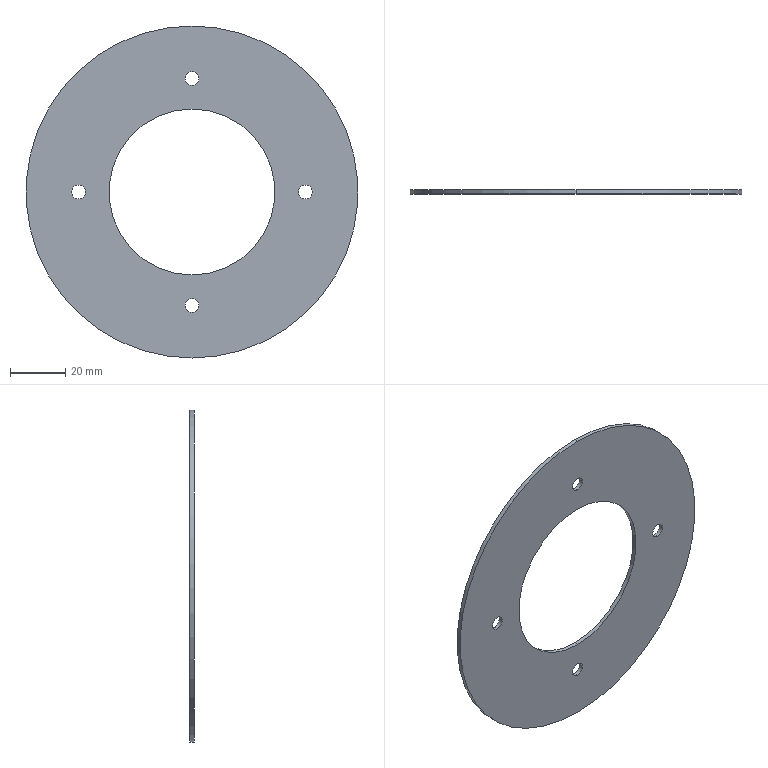Part | SolidWorks | features BaseBody 1 | 1 solid | 14 faces | box 120 x 1.5 x 120 mm | volume 12606 mm3 | cylinder 12 | plane 2 | commonest cylinder face diameters 5 x8 60 x2 120 x2
STEP:
#1=CARTESIAN_POINT('',(0.,1.5,-60.));
#2=VERTEX_POINT('',#1);
#3=CARTESIAN_POINT('',(0.,1.5,60.));
#4=VERTEX_POINT('',#3);
#5=CARTESIAN_POINT('',(0.,1.5,0.));
#6=DIRECTION('',(0.,-1.,0.));
#7=DIRECTION('',(0.,0.,-1.));
#8=AXIS2_PLACEMENT_3D('',#5,#6,#7);
#9=CIRCLE('',#8,60.);
#10=EDGE_CURVE('',#2,#4,#9,.T.);
#11=ORIENTED_EDGE('',*,*,#10,.T.);
#12=CARTESIAN_POINT('',(0.,0.,60.));
#13=VERTEX_POINT('',#12);
#14=CARTESIAN_POINT('',(0.,10.,60.));
#15=DIRECTION('',(0.,-1.,0.));
#16=VECTOR('',#15,1000.);
#17=LINE('',#14,#16);
#18=EDGE_CURVE('',#4,#13,#17,.T.);
#19=ORIENTED_EDGE('',*,*,#18,.T.);
#20=CARTESIAN_POINT('',(0.,0.,-60.));
#21=VERTEX_POINT('',#20);
#22=CARTESIAN_POINT('',(0.,0.,0.));
#23=DIRECTION('',(0.,1.,0.));
#24=DIRECTION('',(0.,0.,-1.));
#25=AXIS2_PLACEMENT_3D('',#22,#23,#24);
#26=CIRCLE('',#25,60.);
#27=EDGE_CURVE('',#13,#21,#26,.T.);
#28=ORIENTED_EDGE('',*,*,#27,.T.);
#29=CARTESIAN_POINT('',(0.,10.,-60.));
#30=DIRECTION('',(0.,-1.,0.));
#31=VECTOR('',#30,1000.);
#32=LINE('',#29,#31);
#33=EDGE_CURVE('',#2,#21,#32,.T.);
#34=ORIENTED_EDGE('',*,*,#33,.F.);
#35=EDGE_LOOP('',(#11,#19,#28,#34));
#36=FACE_OUTER_BOUND('',#35,.T.);
#37=CARTESIAN_POINT('',(0.,10.,0.));
#38=DIRECTION('',(0.,-1.,0.));
#39=DIRECTION('',(0.,0.,-1.));
#40=AXIS2_PLACEMENT_3D('',#37,#38,#39);
#41=CYLINDRICAL_SURFACE('',#40,60.);
#42=ADVANCED_FACE('',(#36),#41,.T.);
#43=CARTESIAN_POINT('',(-41.,1.5,2.5));
#44=VERTEX_POINT('',#43);
#45=CARTESIAN_POINT('',(-41.,1.5,-2.5));
#46=VERTEX_POINT('',#45);
#47=CARTESIAN_POINT('',(-41.,1.5,0.));
#48=DIRECTION('',(0.,-1.,0.));
#49=DIRECTION('',(0.,0.,-1.));
#50=AXIS2_PLACEMENT_3D('',#47,#48,#49);
#51=CIRCLE('',#50,2.5);
#52=EDGE_CURVE('',#44,#46,#51,.T.);
#53=ORIENTED_EDGE('',*,*,#52,.F.);
#54=CARTESIAN_POINT('',(-41.,0.,2.5));
#55=VERTEX_POINT('',#54);
#56=CARTESIAN_POINT('',(-41.,1.5,2.5));
#57=DIRECTION('',(0.,-1.,0.));
#58=VECTOR('',#57,1000.);
#59=LINE('',#56,#58);
#60=EDGE_CURVE('',#44,#55,#59,.T.);
#61=ORIENTED_EDGE('',*,*,#60,.T.);
#62=CARTESIAN_POINT('',(-41.,0.,-2.5));
#63=VERTEX_POINT('',#62);
#64=CARTESIAN_POINT('',(-41.,0.,0.));
#65=DIRECTION('',(0.,-1.,0.));
#66=DIRECTION('',(0.,0.,-1.));
#67=AXIS2_PLACEMENT_3D('',#64,#65,#66);
#68=CIRCLE('',#67,2.5);
#69=EDGE_CURVE('',#55,#63,#68,.T.);
#70=ORIENTED_EDGE('',*,*,#69,.T.);
#71=CARTESIAN_POINT('',(-41.,1.5,-2.5));
#72=DIRECTION('',(0.,-1.,0.));
#73=VECTOR('',#72,1000.);
#74=LINE('',#71,#73);
#75=EDGE_CURVE('',#46,#63,#74,.T.);
#76=ORIENTED_EDGE('',*,*,#75,.F.);
#77=EDGE_LOOP('',(#53,#61,#70,#76));
#78=FACE_OUTER_BOUND('',#77,.T.);
#79=CARTESIAN_POINT('',(-41.,1.5,0.));
#80=DIRECTION('',(0.,-1.,0.));
#81=DIRECTION('',(0.,0.,-1.));
#82=AXIS2_PLACEMENT_3D('',#79,#80,#81);
#83=CYLINDRICAL_SURFACE('',#82,2.5);
#84=ADVANCED_FACE('',(#78),#83,.F.);
#85=CARTESIAN_POINT('',(0.,1.5,43.5));
#86=VERTEX_POINT('',#85);
#87=CARTESIAN_POINT('',(0.,1.5,38.5));
#88=VERTEX_POINT('',#87);
#89=CARTESIAN_POINT('',(0.,1.5,41.));
#90=DIRECTION('',(0.,-1.,0.));
#91=DIRECTION('',(0.,0.,-1.));
#92=AXIS2_PLACEMENT_3D('',#89,#90,#91);
#93=CIRCLE('',#92,2.5);
#94=EDGE_CURVE('',#86,#88,#93,.T.);
#95=ORIENTED_EDGE('',*,*,#94,.F.);
#96=CARTESIAN_POINT('',(0.,0.,43.5));
#97=VERTEX_POINT('',#96);
#98=CARTESIAN_POINT('',(0.,1.5,43.5));
#99=DIRECTION('',(0.,-1.,0.));
#100=VECTOR('',#99,1000.);
#101=LINE('',#98,#100);
#102=EDGE_CURVE('',#86,#97,#101,.T.);
#103=ORIENTED_EDGE('',*,*,#102,.T.);
#104=CARTESIAN_POINT('',(0.,0.,38.5));
#105=VERTEX_POINT('',#104);
#106=CARTESIAN_POINT('',(0.,0.,41.));
#107=DIRECTION('',(0.,-1.,0.));
#108=DIRECTION('',(0.,0.,-1.));
#109=AXIS2_PLACEMENT_3D('',#106,#107,#108);
#110=CIRCLE('',#109,2.5);
#111=EDGE_CURVE('',#97,#105,#110,.T.);
#112=ORIENTED_EDGE('',*,*,#111,.T.);
#113=CARTESIAN_POINT('',(0.,1.5,38.5));
#114=DIRECTION('',(0.,-1.,0.));
#115=VECTOR('',#114,1000.);
#116=LINE('',#113,#115);
#117=EDGE_CURVE('',#88,#105,#116,.T.);
#118=ORIENTED_EDGE('',*,*,#117,.F.);
#119=EDGE_LOOP('',(#95,#103,#112,#118));
#120=FACE_OUTER_BOUND('',#119,.T.);
#121=CARTESIAN_POINT('',(0.,1.5,41.));
#122=DIRECTION('',(0.,-1.,0.));
#123=DIRECTION('',(0.,0.,-1.));
#124=AXIS2_PLACEMENT_3D('',#121,#122,#123);
#125=CYLINDRICAL_SURFACE('',#124,2.5);
#126=ADVANCED_FACE('',(#120),#125,.F.);
#127=CARTESIAN_POINT('',(41.,1.5,2.5));
#128=VERTEX_POINT('',#127);
#129=CARTESIAN_POINT('',(41.,1.5,-2.5));
#130=VERTEX_POINT('',#129);
#131=CARTESIAN_POINT('',(41.,1.5,0.));
#132=DIRECTION('',(0.,-1.,0.));
#133=DIRECTION('',(0.,0.,-1.));
#134=AXIS2_PLACEMENT_3D('',#131,#132,#133);
#135=CIRCLE('',#134,2.5);
#136=EDGE_CURVE('',#128,#130,#135,.T.);
#137=ORIENTED_EDGE('',*,*,#136,.F.);
#138=CARTESIAN_POINT('',(41.,0.,2.5));
#139=VERTEX_POINT('',#138);
#140=CARTESIAN_POINT('',(41.,1.5,2.5));
#141=DIRECTION('',(0.,-1.,0.));
#142=VECTOR('',#141,1000.);
#143=LINE('',#140,#142);
#144=EDGE_CURVE('',#128,#139,#143,.T.);
#145=ORIENTED_EDGE('',*,*,#144,.T.);
#146=CARTESIAN_POINT('',(41.,0.,-2.5));
#147=VERTEX_POINT('',#146);
#148=CARTESIAN_POINT('',(41.,0.,0.));
#149=DIRECTION('',(0.,-1.,0.));
#150=DIRECTION('',(0.,0.,-1.));
#151=AXIS2_PLACEMENT_3D('',#148,#149,#150);
#152=CIRCLE('',#151,2.5);
#153=EDGE_CURVE('',#139,#147,#152,.T.);
#154=ORIENTED_EDGE('',*,*,#153,.T.);
#155=CARTESIAN_POINT('',(41.,1.5,-2.5));
#156=DIRECTION('',(0.,-1.,0.));
#157=VECTOR('',#156,1000.);
#158=LINE('',#155,#157);
#159=EDGE_CURVE('',#130,#147,#158,.T.);
#160=ORIENTED_EDGE('',*,*,#159,.F.);
#161=EDGE_LOOP('',(#137,#145,#154,#160));
#162=FACE_OUTER_BOUND('',#161,.T.);
#163=CARTESIAN_POINT('',(41.,1.5,0.));
#164=DIRECTION('',(0.,-1.,0.));
#165=DIRECTION('',(0.,0.,-1.));
#166=AXIS2_PLACEMENT_3D('',#163,#164,#165);
#167=CYLINDRICAL_SURFACE('',#166,2.5);
#168=ADVANCED_FACE('',(#162),#167,.F.);
#169=CARTESIAN_POINT('',(0.,1.5,-38.5));
#170=VERTEX_POINT('',#169);
#171=CARTESIAN_POINT('',(0.,1.5,-43.5));
#172=VERTEX_POINT('',#171);
#173=CARTESIAN_POINT('',(0.,1.5,-41.));
#174=DIRECTION('',(0.,-1.,0.));
#175=DIRECTION('',(0.,0.,-1.));
#176=AXIS2_PLACEMENT_3D('',#173,#174,#175);
#177=CIRCLE('',#176,2.5);
#178=EDGE_CURVE('',#170,#172,#177,.T.);
#179=ORIENTED_EDGE('',*,*,#178,.F.);
#180=CARTESIAN_POINT('',(0.,0.,-38.5));
#181=VERTEX_POINT('',#180);
#182=CARTESIAN_POINT('',(0.,1.5,-38.5));
#183=DIRECTION('',(0.,-1.,0.));
#184=VECTOR('',#183,1000.);
#185=LINE('',#182,#184);
#186=EDGE_CURVE('',#170,#181,#185,.T.);
#187=ORIENTED_EDGE('',*,*,#186,.T.);
#188=CARTESIAN_POINT('',(0.,0.,-43.5));
#189=VERTEX_POINT('',#188);
#190=CARTESIAN_POINT('',(0.,0.,-41.));
#191=DIRECTION('',(0.,-1.,0.));
#192=DIRECTION('',(0.,0.,-1.));
#193=AXIS2_PLACEMENT_3D('',#190,#191,#192);
#194=CIRCLE('',#193,2.5);
#195=EDGE_CURVE('',#181,#189,#194,.T.);
#196=ORIENTED_EDGE('',*,*,#195,.T.);
#197=CARTESIAN_POINT('',(0.,1.5,-43.5));
#198=DIRECTION('',(0.,-1.,0.));
#199=VECTOR('',#198,1000.);
#200=LINE('',#197,#199);
#201=EDGE_CURVE('',#172,#189,#200,.T.);
#202=ORIENTED_EDGE('',*,*,#201,.F.);
#203=EDGE_LOOP('',(#179,#187,#196,#202));
#204=FACE_OUTER_BOUND('',#203,.T.);
#205=CARTESIAN_POINT('',(0.,1.5,-41.));
#206=DIRECTION('',(0.,-1.,0.));
#207=DIRECTION('',(0.,0.,-1.));
#208=AXIS2_PLACEMENT_3D('',#205,#206,#207);
#209=CYLINDRICAL_SURFACE('',#208,2.5);
#210=ADVANCED_FACE('',(#204),#209,.F.);
#211=CARTESIAN_POINT('',(0.,1.5,30.));
#212=VERTEX_POINT('',#211);
#213=CARTESIAN_POINT('',(0.,1.5,-30.));
#214=VERTEX_POINT('',#213);
#215=CARTESIAN_POINT('',(0.,1.5,0.));
#216=DIRECTION('',(0.,-1.,0.));
#217=DIRECTION('',(0.,0.,-1.));
#218=AXIS2_PLACEMENT_3D('',#215,#216,#217);
#219=CIRCLE('',#218,30.);
#220=EDGE_CURVE('',#212,#214,#219,.T.);
#221=ORIENTED_EDGE('',*,*,#220,.F.);
#222=CARTESIAN_POINT('',(0.,0.,30.));
#223=VERTEX_POINT('',#222);
#224=CARTESIAN_POINT('',(0.,10.,30.));
#225=DIRECTION('',(0.,-1.,0.));
#226=VECTOR('',#225,1000.);
#227=LINE('',#224,#226);
#228=EDGE_CURVE('',#212,#223,#227,.T.);
#229=ORIENTED_EDGE('',*,*,#228,.T.);
#230=CARTESIAN_POINT('',(0.,0.,-30.));
#231=VERTEX_POINT('',#230);
#232=CARTESIAN_POINT('',(0.,0.,0.));
#233=DIRECTION('',(0.,-1.,0.));
#234=DIRECTION('',(0.,0.,-1.));
#235=AXIS2_PLACEMENT_3D('',#232,#233,#234);
#236=CIRCLE('',#235,30.);
#237=EDGE_CURVE('',#223,#231,#236,.T.);
#238=ORIENTED_EDGE('',*,*,#237,.T.);
#239=CARTESIAN_POINT('',(0.,10.,-30.));
#240=DIRECTION('',(0.,-1.,0.));
#241=VECTOR('',#240,1000.);
#242=LINE('',#239,#241);
#243=EDGE_CURVE('',#214,#231,#242,.T.);
#244=ORIENTED_EDGE('',*,*,#243,.F.);
#245=EDGE_LOOP('',(#221,#229,#238,#244));
#246=FACE_OUTER_BOUND('',#245,.T.);
#247=CARTESIAN_POINT('',(0.,10.,0.));
#248=DIRECTION('',(0.,-1.,0.));
#249=DIRECTION('',(0.,0.,-1.));
#250=AXIS2_PLACEMENT_3D('',#247,#248,#249);
#251=CYLINDRICAL_SURFACE('',#250,30.);
#252=ADVANCED_FACE('',(#246),#251,.F.);
#253=CARTESIAN_POINT('',(0.,0.,0.));
#254=DIRECTION('',(0.,1.,0.));
#255=DIRECTION('',(0.,0.,-1.));
#256=AXIS2_PLACEMENT_3D('',#253,#254,#255);
#257=CIRCLE('',#256,60.);
#258=EDGE_CURVE('',#21,#13,#257,.T.);
#259=ORIENTED_EDGE('',*,*,#258,.F.);
#260=ORIENTED_EDGE('',*,*,#27,.F.);
#261=EDGE_LOOP('',(#259,#260));
#262=FACE_OUTER_BOUND('',#261,.T.);
#263=CARTESIAN_POINT('',(-41.,0.,0.));
#264=DIRECTION('',(0.,-1.,0.));
#265=DIRECTION('',(0.,0.,-1.));
#266=AXIS2_PLACEMENT_3D('',#263,#264,#265);
#267=CIRCLE('',#266,2.5);
#268=EDGE_CURVE('',#63,#55,#267,.T.);
#269=ORIENTED_EDGE('',*,*,#268,.F.);
#270=ORIENTED_EDGE('',*,*,#69,.F.);
#271=EDGE_LOOP('',(#269,#270));
#272=FACE_BOUND('',#271,.T.);
#273=CARTESIAN_POINT('',(0.,0.,41.));
#274=DIRECTION('',(0.,-1.,0.));
#275=DIRECTION('',(0.,0.,-1.));
#276=AXIS2_PLACEMENT_3D('',#273,#274,#275);
#277=CIRCLE('',#276,2.5);
#278=EDGE_CURVE('',#105,#97,#277,.T.);
#279=ORIENTED_EDGE('',*,*,#278,.F.);
#280=ORIENTED_EDGE('',*,*,#111,.F.);
#281=EDGE_LOOP('',(#279,#280));
#282=FACE_BOUND('',#281,.T.);
#283=CARTESIAN_POINT('',(41.,0.,0.));
#284=DIRECTION('',(0.,-1.,0.));
#285=DIRECTION('',(0.,0.,-1.));
#286=AXIS2_PLACEMENT_3D('',#283,#284,#285);
#287=CIRCLE('',#286,2.5);
#288=EDGE_CURVE('',#147,#139,#287,.T.);
#289=ORIENTED_EDGE('',*,*,#288,.F.);
#290=ORIENTED_EDGE('',*,*,#153,.F.);
#291=EDGE_LOOP('',(#289,#290));
#292=FACE_BOUND('',#291,.T.);
#293=CARTESIAN_POINT('',(0.,0.,-41.));
#294=DIRECTION('',(0.,-1.,0.));
#295=DIRECTION('',(0.,0.,-1.));
#296=AXIS2_PLACEMENT_3D('',#293,#294,#295);
#297=CIRCLE('',#296,2.5);
#298=EDGE_CURVE('',#189,#181,#297,.T.);
#299=ORIENTED_EDGE('',*,*,#298,.F.);
#300=ORIENTED_EDGE('',*,*,#195,.F.);
#301=EDGE_LOOP('',(#299,#300));
#302=FACE_BOUND('',#301,.T.);
#303=CARTESIAN_POINT('',(0.,0.,0.));
#304=DIRECTION('',(0.,-1.,0.));
#305=DIRECTION('',(0.,0.,-1.));
#306=AXIS2_PLACEMENT_3D('',#303,#304,#305);
#307=CIRCLE('',#306,30.);
#308=EDGE_CURVE('',#231,#223,#307,.T.);
#309=ORIENTED_EDGE('',*,*,#308,.F.);
#310=ORIENTED_EDGE('',*,*,#237,.F.);
#311=EDGE_LOOP('',(#309,#310));
#312=FACE_BOUND('',#311,.T.);
#313=CARTESIAN_POINT('',(0.,0.,0.));
#314=DIRECTION('',(0.,1.,0.));
#315=DIRECTION('',(0.,0.,1.));
#316=AXIS2_PLACEMENT_3D('',#313,#314,#315);
#317=PLANE('',#316);
#318=ADVANCED_FACE('',(#262,#272,#282,#292,#302,#312),#317,.F.);
#319=ORIENTED_EDGE('',*,*,#18,.F.);
#320=CARTESIAN_POINT('',(0.,1.5,0.));
#321=DIRECTION('',(0.,-1.,0.));
#322=DIRECTION('',(0.,0.,-1.));
#323=AXIS2_PLACEMENT_3D('',#320,#321,#322);
#324=CIRCLE('',#323,60.);
#325=EDGE_CURVE('',#4,#2,#324,.T.);
#326=ORIENTED_EDGE('',*,*,#325,.T.);
#327=ORIENTED_EDGE('',*,*,#33,.T.);
#328=ORIENTED_EDGE('',*,*,#258,.T.);
#329=EDGE_LOOP('',(#319,#326,#327,#328));
#330=FACE_OUTER_BOUND('',#329,.T.);
#331=CARTESIAN_POINT('',(0.,10.,0.));
#332=DIRECTION('',(0.,-1.,0.));
#333=DIRECTION('',(0.,0.,-1.));
#334=AXIS2_PLACEMENT_3D('',#331,#332,#333);
#335=CYLINDRICAL_SURFACE('',#334,60.);
#336=ADVANCED_FACE('',(#330),#335,.T.);
#337=ORIENTED_EDGE('',*,*,#60,.F.);
#338=CARTESIAN_POINT('',(-41.,1.5,0.));
#339=DIRECTION('',(0.,-1.,0.));
#340=DIRECTION('',(0.,0.,-1.));
#341=AXIS2_PLACEMENT_3D('',#338,#339,#340);
#342=CIRCLE('',#341,2.5);
#343=EDGE_CURVE('',#46,#44,#342,.T.);
#344=ORIENTED_EDGE('',*,*,#343,.F.);
#345=ORIENTED_EDGE('',*,*,#75,.T.);
#346=ORIENTED_EDGE('',*,*,#268,.T.);
#347=EDGE_LOOP('',(#337,#344,#345,#346));
#348=FACE_OUTER_BOUND('',#347,.T.);
#349=CARTESIAN_POINT('',(-41.,1.5,0.));
#350=DIRECTION('',(0.,-1.,0.));
#351=DIRECTION('',(0.,0.,-1.));
#352=AXIS2_PLACEMENT_3D('',#349,#350,#351);
#353=CYLINDRICAL_SURFACE('',#352,2.5);
#354=ADVANCED_FACE('',(#348),#353,.F.);
#355=ORIENTED_EDGE('',*,*,#102,.F.);
#356=CARTESIAN_POINT('',(0.,1.5,41.));
#357=DIRECTION('',(0.,-1.,0.));
#358=DIRECTION('',(0.,0.,-1.));
#359=AXIS2_PLACEMENT_3D('',#356,#357,#358);
#360=CIRCLE('',#359,2.5);
#361=EDGE_CURVE('',#88,#86,#360,.T.);
#362=ORIENTED_EDGE('',*,*,#361,.F.);
#363=ORIENTED_EDGE('',*,*,#117,.T.);
#364=ORIENTED_EDGE('',*,*,#278,.T.);
#365=EDGE_LOOP('',(#355,#362,#363,#364));
#366=FACE_OUTER_BOUND('',#365,.T.);
#367=CARTESIAN_POINT('',(0.,1.5,41.));
#368=DIRECTION('',(0.,-1.,0.));
#369=DIRECTION('',(0.,0.,-1.));
#370=AXIS2_PLACEMENT_3D('',#367,#368,#369);
#371=CYLINDRICAL_SURFACE('',#370,2.5);
#372=ADVANCED_FACE('',(#366),#371,.F.);
#373=ORIENTED_EDGE('',*,*,#144,.F.);
#374=CARTESIAN_POINT('',(41.,1.5,0.));
#375=DIRECTION('',(0.,-1.,0.));
#376=DIRECTION('',(0.,0.,-1.));
#377=AXIS2_PLACEMENT_3D('',#374,#375,#376);
#378=CIRCLE('',#377,2.5);
#379=EDGE_CURVE('',#130,#128,#378,.T.);
#380=ORIENTED_EDGE('',*,*,#379,.F.);
#381=ORIENTED_EDGE('',*,*,#159,.T.);
#382=ORIENTED_EDGE('',*,*,#288,.T.);
#383=EDGE_LOOP('',(#373,#380,#381,#382));
#384=FACE_OUTER_BOUND('',#383,.T.);
#385=CARTESIAN_POINT('',(41.,1.5,0.));
#386=DIRECTION('',(0.,-1.,0.));
#387=DIRECTION('',(0.,0.,-1.));
#388=AXIS2_PLACEMENT_3D('',#385,#386,#387);
#389=CYLINDRICAL_SURFACE('',#388,2.5);
#390=ADVANCED_FACE('',(#384),#389,.F.);
#391=ORIENTED_EDGE('',*,*,#186,.F.);
#392=CARTESIAN_POINT('',(0.,1.5,-41.));
#393=DIRECTION('',(0.,-1.,0.));
#394=DIRECTION('',(0.,0.,-1.));
#395=AXIS2_PLACEMENT_3D('',#392,#393,#394);
#396=CIRCLE('',#395,2.5);
#397=EDGE_CURVE('',#172,#170,#396,.T.);
#398=ORIENTED_EDGE('',*,*,#397,.F.);
#399=ORIENTED_EDGE('',*,*,#201,.T.);
#400=ORIENTED_EDGE('',*,*,#298,.T.);
#401=EDGE_LOOP('',(#391,#398,#399,#400));
#402=FACE_OUTER_BOUND('',#401,.T.);
#403=CARTESIAN_POINT('',(0.,1.5,-41.));
#404=DIRECTION('',(0.,-1.,0.));
#405=DIRECTION('',(0.,0.,-1.));
#406=AXIS2_PLACEMENT_3D('',#403,#404,#405);
#407=CYLINDRICAL_SURFACE('',#406,2.5);
#408=ADVANCED_FACE('',(#402),#407,.F.);
#409=ORIENTED_EDGE('',*,*,#228,.F.);
#410=CARTESIAN_POINT('',(0.,1.5,0.));
#411=DIRECTION('',(0.,-1.,0.));
#412=DIRECTION('',(0.,0.,-1.));
#413=AXIS2_PLACEMENT_3D('',#410,#411,#412);
#414=CIRCLE('',#413,30.);
#415=EDGE_CURVE('',#214,#212,#414,.T.);
#416=ORIENTED_EDGE('',*,*,#415,.F.);
#417=ORIENTED_EDGE('',*,*,#243,.T.);
#418=ORIENTED_EDGE('',*,*,#308,.T.);
#419=EDGE_LOOP('',(#409,#416,#417,#418));
#420=FACE_OUTER_BOUND('',#419,.T.);
#421=CARTESIAN_POINT('',(0.,10.,0.));
#422=DIRECTION('',(0.,-1.,0.));
#423=DIRECTION('',(0.,0.,-1.));
#424=AXIS2_PLACEMENT_3D('',#421,#422,#423);
#425=CYLINDRICAL_SURFACE('',#424,30.);
#426=ADVANCED_FACE('',(#420),#425,.F.);
#427=ORIENTED_EDGE('',*,*,#10,.F.);
#428=ORIENTED_EDGE('',*,*,#325,.F.);
#429=EDGE_LOOP('',(#427,#428));
#430=FACE_OUTER_BOUND('',#429,.T.);
#431=ORIENTED_EDGE('',*,*,#343,.T.);
#432=ORIENTED_EDGE('',*,*,#52,.T.);
#433=EDGE_LOOP('',(#431,#432));
#434=FACE_BOUND('',#433,.T.);
#435=ORIENTED_EDGE('',*,*,#379,.T.);
#436=ORIENTED_EDGE('',*,*,#136,.T.);
#437=EDGE_LOOP('',(#435,#436));
#438=FACE_BOUND('',#437,.T.);
#439=ORIENTED_EDGE('',*,*,#397,.T.);
#440=ORIENTED_EDGE('',*,*,#178,.T.);
#441=EDGE_LOOP('',(#439,#440));
#442=FACE_BOUND('',#441,.T.);
#443=ORIENTED_EDGE('',*,*,#361,.T.);
#444=ORIENTED_EDGE('',*,*,#94,.T.);
#445=EDGE_LOOP('',(#443,#444));
#446=FACE_BOUND('',#445,.T.);
#447=ORIENTED_EDGE('',*,*,#415,.T.);
#448=ORIENTED_EDGE('',*,*,#220,.T.);
#449=EDGE_LOOP('',(#447,#448));
#450=FACE_BOUND('',#449,.T.);
#451=CARTESIAN_POINT('',(0.,1.5,0.));
#452=DIRECTION('',(0.,1.,0.));
#453=DIRECTION('',(0.,0.,1.));
#454=AXIS2_PLACEMENT_3D('',#451,#452,#453);
#455=PLANE('',#454);
#456=ADVANCED_FACE('',(#430,#434,#438,#442,#446,#450),#455,.T.);
#457=CLOSED_SHELL('',(#42,#84,#126,#168,#210,#252,#318,#336,#354,#372,#390,#408,#426,#456));
#458=MANIFOLD_SOLID_BREP('',#457);
#459=CARTESIAN_POINT('',(0.,0.,0.));
#460=DIRECTION('',(0.,0.,1.));
#461=DIRECTION('',(1.,0.,0.));
#462=AXIS2_PLACEMENT_3D('',#459,#460,#461);
#463=(LENGTH_UNIT()NAMED_UNIT(*)SI_UNIT(.MILLI.,.METRE.));
#464=UNCERTAINTY_MEASURE_WITH_UNIT(LENGTH_MEASURE(0.00001),#463,'','');
#465=(NAMED_UNIT(*)PLANE_ANGLE_UNIT()SI_UNIT($,.RADIAN.));
#466=(NAMED_UNIT(*)SI_UNIT($,.STERADIAN.)SOLID_ANGLE_UNIT());
#467=(GEOMETRIC_REPRESENTATION_CONTEXT(3)GLOBAL_UNCERTAINTY_ASSIGNED_CONTEXT((#464))GLOBAL_UNIT_ASSIGNED_CONTEXT((#463,#465,#466))REPRESENTATION_CONTEXT('',''));
#468=ADVANCED_BREP_SHAPE_REPRESENTATION('',(#458,#462),#467);